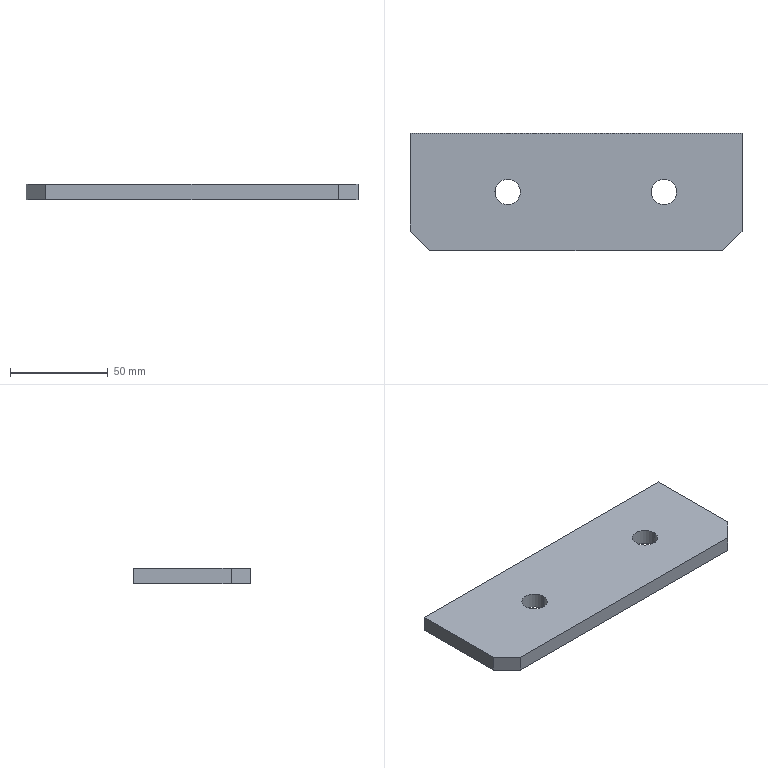Part | SolidWorks | features Extrusion 1, ICE 1 | 1 solid | 12 faces | box 170 x 60 x 8 mm | volume 78676 mm3 | plane 8 | cylinder 4 | commonest cylinder face diameters 13 x4
STEP:
#1=CARTESIAN_POINT('',(123.5,30.,0.));
#2=VERTEX_POINT('',#1);
#3=CARTESIAN_POINT('',(136.5,30.,0.));
#4=VERTEX_POINT('',#3);
#5=CARTESIAN_POINT('',(130.,30.,0.));
#6=DIRECTION('',(0.,0.,1.));
#7=DIRECTION('',(1.,0.,0.));
#8=AXIS2_PLACEMENT_3D('',#5,#6,#7);
#9=CIRCLE('',#8,6.5);
#10=EDGE_CURVE('',#2,#4,#9,.T.);
#11=ORIENTED_EDGE('',*,*,#10,.F.);
#12=CARTESIAN_POINT('',(123.5,30.,8.));
#13=VERTEX_POINT('',#12);
#14=CARTESIAN_POINT('',(123.5,30.,0.));
#15=DIRECTION('',(0.,0.,1.));
#16=VECTOR('',#15,1000.);
#17=LINE('',#14,#16);
#18=EDGE_CURVE('',#2,#13,#17,.T.);
#19=ORIENTED_EDGE('',*,*,#18,.T.);
#20=CARTESIAN_POINT('',(136.5,30.,8.));
#21=VERTEX_POINT('',#20);
#22=CARTESIAN_POINT('',(130.,30.,8.));
#23=DIRECTION('',(0.,0.,1.));
#24=DIRECTION('',(1.,0.,0.));
#25=AXIS2_PLACEMENT_3D('',#22,#23,#24);
#26=CIRCLE('',#25,6.5);
#27=EDGE_CURVE('',#13,#21,#26,.T.);
#28=ORIENTED_EDGE('',*,*,#27,.T.);
#29=CARTESIAN_POINT('',(136.5,30.,0.));
#30=DIRECTION('',(0.,0.,1.));
#31=VECTOR('',#30,1000.);
#32=LINE('',#29,#31);
#33=EDGE_CURVE('',#4,#21,#32,.T.);
#34=ORIENTED_EDGE('',*,*,#33,.F.);
#35=EDGE_LOOP('',(#11,#19,#28,#34));
#36=FACE_OUTER_BOUND('',#35,.T.);
#37=CARTESIAN_POINT('',(130.,30.,0.));
#38=DIRECTION('',(0.,0.,1.));
#39=DIRECTION('',(1.,0.,0.));
#40=AXIS2_PLACEMENT_3D('',#37,#38,#39);
#41=CYLINDRICAL_SURFACE('',#40,6.5);
#42=ADVANCED_FACE('',(#36),#41,.F.);
#43=CARTESIAN_POINT('',(43.5,30.,0.));
#44=VERTEX_POINT('',#43);
#45=CARTESIAN_POINT('',(56.5,30.,0.));
#46=VERTEX_POINT('',#45);
#47=CARTESIAN_POINT('',(50.,30.,0.));
#48=DIRECTION('',(0.,0.,1.));
#49=DIRECTION('',(1.,0.,0.));
#50=AXIS2_PLACEMENT_3D('',#47,#48,#49);
#51=CIRCLE('',#50,6.5);
#52=EDGE_CURVE('',#44,#46,#51,.T.);
#53=ORIENTED_EDGE('',*,*,#52,.F.);
#54=CARTESIAN_POINT('',(43.5,30.,8.));
#55=VERTEX_POINT('',#54);
#56=CARTESIAN_POINT('',(43.5,30.,0.));
#57=DIRECTION('',(0.,0.,1.));
#58=VECTOR('',#57,1000.);
#59=LINE('',#56,#58);
#60=EDGE_CURVE('',#44,#55,#59,.T.);
#61=ORIENTED_EDGE('',*,*,#60,.T.);
#62=CARTESIAN_POINT('',(56.5,30.,8.));
#63=VERTEX_POINT('',#62);
#64=CARTESIAN_POINT('',(50.,30.,8.));
#65=DIRECTION('',(0.,0.,1.));
#66=DIRECTION('',(1.,0.,0.));
#67=AXIS2_PLACEMENT_3D('',#64,#65,#66);
#68=CIRCLE('',#67,6.5);
#69=EDGE_CURVE('',#55,#63,#68,.T.);
#70=ORIENTED_EDGE('',*,*,#69,.T.);
#71=CARTESIAN_POINT('',(56.5,30.,0.));
#72=DIRECTION('',(0.,0.,1.));
#73=VECTOR('',#72,1000.);
#74=LINE('',#71,#73);
#75=EDGE_CURVE('',#46,#63,#74,.T.);
#76=ORIENTED_EDGE('',*,*,#75,.F.);
#77=EDGE_LOOP('',(#53,#61,#70,#76));
#78=FACE_OUTER_BOUND('',#77,.T.);
#79=CARTESIAN_POINT('',(50.,30.,0.));
#80=DIRECTION('',(0.,0.,1.));
#81=DIRECTION('',(1.,0.,0.));
#82=AXIS2_PLACEMENT_3D('',#79,#80,#81);
#83=CYLINDRICAL_SURFACE('',#82,6.5);
#84=ADVANCED_FACE('',(#78),#83,.F.);
#85=CARTESIAN_POINT('',(170.,60.,0.));
#86=VERTEX_POINT('',#85);
#87=CARTESIAN_POINT('',(0.,60.,0.));
#88=VERTEX_POINT('',#87);
#89=CARTESIAN_POINT('',(170.,60.,0.));
#90=DIRECTION('',(-1.,0.,0.));
#91=VECTOR('',#90,1000.);
#92=LINE('',#89,#91);
#93=EDGE_CURVE('',#86,#88,#92,.T.);
#94=ORIENTED_EDGE('',*,*,#93,.T.);
#95=CARTESIAN_POINT('',(0.,60.,8.));
#96=VERTEX_POINT('',#95);
#97=CARTESIAN_POINT('',(0.,60.,8.));
#98=DIRECTION('',(0.,0.,-1.));
#99=VECTOR('',#98,1000.);
#100=LINE('',#97,#99);
#101=EDGE_CURVE('',#96,#88,#100,.T.);
#102=ORIENTED_EDGE('',*,*,#101,.F.);
#103=CARTESIAN_POINT('',(170.,60.,8.));
#104=VERTEX_POINT('',#103);
#105=CARTESIAN_POINT('',(170.,60.,8.));
#106=DIRECTION('',(-1.,0.,0.));
#107=VECTOR('',#106,1000.);
#108=LINE('',#105,#107);
#109=EDGE_CURVE('',#104,#96,#108,.T.);
#110=ORIENTED_EDGE('',*,*,#109,.F.);
#111=CARTESIAN_POINT('',(170.,60.,8.));
#112=DIRECTION('',(0.,0.,-1.));
#113=VECTOR('',#112,1000.);
#114=LINE('',#111,#113);
#115=EDGE_CURVE('',#104,#86,#114,.T.);
#116=ORIENTED_EDGE('',*,*,#115,.T.);
#117=EDGE_LOOP('',(#94,#102,#110,#116));
#118=FACE_OUTER_BOUND('',#117,.T.);
#119=CARTESIAN_POINT('',(170.,60.,8.));
#120=DIRECTION('',(0.,-1.,0.));
#121=DIRECTION('',(0.,0.,-1.));
#122=AXIS2_PLACEMENT_3D('',#119,#120,#121);
#123=PLANE('',#122);
#124=ADVANCED_FACE('',(#118),#123,.F.);
#125=CARTESIAN_POINT('',(0.,10.,0.));
#126=VERTEX_POINT('',#125);
#127=CARTESIAN_POINT('',(0.,60.,0.));
#128=DIRECTION('',(0.,-1.,0.));
#129=VECTOR('',#128,1000.);
#130=LINE('',#127,#129);
#131=EDGE_CURVE('',#88,#126,#130,.T.);
#132=ORIENTED_EDGE('',*,*,#131,.T.);
#133=CARTESIAN_POINT('',(0.,10.,8.));
#134=VERTEX_POINT('',#133);
#135=CARTESIAN_POINT('',(0.,10.,8.));
#136=DIRECTION('',(0.,0.,-1.));
#137=VECTOR('',#136,1000.);
#138=LINE('',#135,#137);
#139=EDGE_CURVE('',#134,#126,#138,.T.);
#140=ORIENTED_EDGE('',*,*,#139,.F.);
#141=CARTESIAN_POINT('',(0.,60.,8.));
#142=DIRECTION('',(0.,-1.,0.));
#143=VECTOR('',#142,1000.);
#144=LINE('',#141,#143);
#145=EDGE_CURVE('',#96,#134,#144,.T.);
#146=ORIENTED_EDGE('',*,*,#145,.F.);
#147=ORIENTED_EDGE('',*,*,#101,.T.);
#148=EDGE_LOOP('',(#132,#140,#146,#147));
#149=FACE_OUTER_BOUND('',#148,.T.);
#150=CARTESIAN_POINT('',(0.,60.,8.));
#151=DIRECTION('',(1.,0.,0.));
#152=DIRECTION('',(0.,0.,-1.));
#153=AXIS2_PLACEMENT_3D('',#150,#151,#152);
#154=PLANE('',#153);
#155=ADVANCED_FACE('',(#149),#154,.F.);
#156=CARTESIAN_POINT('',(10.,0.,0.));
#157=VERTEX_POINT('',#156);
#158=CARTESIAN_POINT('',(0.,10.,0.));
#159=DIRECTION('',(0.7071,-0.7071,0.));
#160=VECTOR('',#159,1000.);
#161=LINE('',#158,#160);
#162=EDGE_CURVE('',#126,#157,#161,.T.);
#163=ORIENTED_EDGE('',*,*,#162,.T.);
#164=CARTESIAN_POINT('',(10.,0.,8.));
#165=VERTEX_POINT('',#164);
#166=CARTESIAN_POINT('',(10.,0.,8.));
#167=DIRECTION('',(0.,0.,-1.));
#168=VECTOR('',#167,1000.);
#169=LINE('',#166,#168);
#170=EDGE_CURVE('',#165,#157,#169,.T.);
#171=ORIENTED_EDGE('',*,*,#170,.F.);
#172=CARTESIAN_POINT('',(0.,10.,8.));
#173=DIRECTION('',(0.7071,-0.7071,0.));
#174=VECTOR('',#173,1000.);
#175=LINE('',#172,#174);
#176=EDGE_CURVE('',#134,#165,#175,.T.);
#177=ORIENTED_EDGE('',*,*,#176,.F.);
#178=ORIENTED_EDGE('',*,*,#139,.T.);
#179=EDGE_LOOP('',(#163,#171,#177,#178));
#180=FACE_OUTER_BOUND('',#179,.T.);
#181=CARTESIAN_POINT('',(0.,10.,8.));
#182=DIRECTION('',(0.7071,0.7071,0.));
#183=DIRECTION('',(-0.7071,0.7071,0.));
#184=AXIS2_PLACEMENT_3D('',#181,#182,#183);
#185=PLANE('',#184);
#186=ADVANCED_FACE('',(#180),#185,.F.);
#187=CARTESIAN_POINT('',(160.,0.,0.));
#188=VERTEX_POINT('',#187);
#189=CARTESIAN_POINT('',(10.,0.,0.));
#190=DIRECTION('',(1.,0.,0.));
#191=VECTOR('',#190,1000.);
#192=LINE('',#189,#191);
#193=EDGE_CURVE('',#157,#188,#192,.T.);
#194=ORIENTED_EDGE('',*,*,#193,.T.);
#195=CARTESIAN_POINT('',(160.,0.,8.));
#196=VERTEX_POINT('',#195);
#197=CARTESIAN_POINT('',(160.,0.,8.));
#198=DIRECTION('',(0.,0.,-1.));
#199=VECTOR('',#198,1000.);
#200=LINE('',#197,#199);
#201=EDGE_CURVE('',#196,#188,#200,.T.);
#202=ORIENTED_EDGE('',*,*,#201,.F.);
#203=CARTESIAN_POINT('',(10.,0.,8.));
#204=DIRECTION('',(1.,0.,0.));
#205=VECTOR('',#204,1000.);
#206=LINE('',#203,#205);
#207=EDGE_CURVE('',#165,#196,#206,.T.);
#208=ORIENTED_EDGE('',*,*,#207,.F.);
#209=ORIENTED_EDGE('',*,*,#170,.T.);
#210=EDGE_LOOP('',(#194,#202,#208,#209));
#211=FACE_OUTER_BOUND('',#210,.T.);
#212=CARTESIAN_POINT('',(10.,0.,8.));
#213=DIRECTION('',(0.,1.,0.));
#214=DIRECTION('',(0.,0.,1.));
#215=AXIS2_PLACEMENT_3D('',#212,#213,#214);
#216=PLANE('',#215);
#217=ADVANCED_FACE('',(#211),#216,.F.);
#218=CARTESIAN_POINT('',(170.,10.,0.));
#219=VERTEX_POINT('',#218);
#220=CARTESIAN_POINT('',(160.,0.,0.));
#221=DIRECTION('',(0.7071,0.7071,0.));
#222=VECTOR('',#221,1000.);
#223=LINE('',#220,#222);
#224=EDGE_CURVE('',#188,#219,#223,.T.);
#225=ORIENTED_EDGE('',*,*,#224,.T.);
#226=CARTESIAN_POINT('',(170.,10.,8.));
#227=VERTEX_POINT('',#226);
#228=CARTESIAN_POINT('',(170.,10.,8.));
#229=DIRECTION('',(0.,0.,-1.));
#230=VECTOR('',#229,1000.);
#231=LINE('',#228,#230);
#232=EDGE_CURVE('',#227,#219,#231,.T.);
#233=ORIENTED_EDGE('',*,*,#232,.F.);
#234=CARTESIAN_POINT('',(160.,0.,8.));
#235=DIRECTION('',(0.7071,0.7071,0.));
#236=VECTOR('',#235,1000.);
#237=LINE('',#234,#236);
#238=EDGE_CURVE('',#196,#227,#237,.T.);
#239=ORIENTED_EDGE('',*,*,#238,.F.);
#240=ORIENTED_EDGE('',*,*,#201,.T.);
#241=EDGE_LOOP('',(#225,#233,#239,#240));
#242=FACE_OUTER_BOUND('',#241,.T.);
#243=CARTESIAN_POINT('',(160.,0.,8.));
#244=DIRECTION('',(-0.7071,0.7071,0.));
#245=DIRECTION('',(-0.7071,-0.7071,0.));
#246=AXIS2_PLACEMENT_3D('',#243,#244,#245);
#247=PLANE('',#246);
#248=ADVANCED_FACE('',(#242),#247,.F.);
#249=CARTESIAN_POINT('',(170.,10.,0.));
#250=DIRECTION('',(0.,1.,0.));
#251=VECTOR('',#250,1000.);
#252=LINE('',#249,#251);
#253=EDGE_CURVE('',#219,#86,#252,.T.);
#254=ORIENTED_EDGE('',*,*,#253,.T.);
#255=ORIENTED_EDGE('',*,*,#115,.F.);
#256=CARTESIAN_POINT('',(170.,10.,8.));
#257=DIRECTION('',(0.,1.,0.));
#258=VECTOR('',#257,1000.);
#259=LINE('',#256,#258);
#260=EDGE_CURVE('',#227,#104,#259,.T.);
#261=ORIENTED_EDGE('',*,*,#260,.F.);
#262=ORIENTED_EDGE('',*,*,#232,.T.);
#263=EDGE_LOOP('',(#254,#255,#261,#262));
#264=FACE_OUTER_BOUND('',#263,.T.);
#265=CARTESIAN_POINT('',(170.,10.,8.));
#266=DIRECTION('',(-1.,0.,0.));
#267=DIRECTION('',(0.,0.,1.));
#268=AXIS2_PLACEMENT_3D('',#265,#266,#267);
#269=PLANE('',#268);
#270=ADVANCED_FACE('',(#264),#269,.F.);
#271=CARTESIAN_POINT('',(130.,30.,8.));
#272=DIRECTION('',(0.,0.,1.));
#273=DIRECTION('',(1.,0.,0.));
#274=AXIS2_PLACEMENT_3D('',#271,#272,#273);
#275=CIRCLE('',#274,6.5);
#276=EDGE_CURVE('',#21,#13,#275,.T.);
#277=ORIENTED_EDGE('',*,*,#276,.F.);
#278=ORIENTED_EDGE('',*,*,#27,.F.);
#279=EDGE_LOOP('',(#277,#278));
#280=FACE_BOUND('',#279,.T.);
#281=CARTESIAN_POINT('',(50.,30.,8.));
#282=DIRECTION('',(0.,0.,1.));
#283=DIRECTION('',(1.,0.,0.));
#284=AXIS2_PLACEMENT_3D('',#281,#282,#283);
#285=CIRCLE('',#284,6.5);
#286=EDGE_CURVE('',#63,#55,#285,.T.);
#287=ORIENTED_EDGE('',*,*,#286,.F.);
#288=ORIENTED_EDGE('',*,*,#69,.F.);
#289=EDGE_LOOP('',(#287,#288));
#290=FACE_BOUND('',#289,.T.);
#291=ORIENTED_EDGE('',*,*,#109,.T.);
#292=ORIENTED_EDGE('',*,*,#145,.T.);
#293=ORIENTED_EDGE('',*,*,#176,.T.);
#294=ORIENTED_EDGE('',*,*,#207,.T.);
#295=ORIENTED_EDGE('',*,*,#238,.T.);
#296=ORIENTED_EDGE('',*,*,#260,.T.);
#297=EDGE_LOOP('',(#291,#292,#293,#294,#295,#296));
#298=FACE_OUTER_BOUND('',#297,.T.);
#299=CARTESIAN_POINT('',(0.,0.,8.));
#300=DIRECTION('',(0.,0.,1.));
#301=DIRECTION('',(1.,0.,0.));
#302=AXIS2_PLACEMENT_3D('',#299,#300,#301);
#303=PLANE('',#302);
#304=ADVANCED_FACE('',(#280,#290,#298),#303,.T.);
#305=CARTESIAN_POINT('',(130.,30.,0.));
#306=DIRECTION('',(0.,0.,1.));
#307=DIRECTION('',(1.,0.,0.));
#308=AXIS2_PLACEMENT_3D('',#305,#306,#307);
#309=CIRCLE('',#308,6.5);
#310=EDGE_CURVE('',#4,#2,#309,.T.);
#311=ORIENTED_EDGE('',*,*,#310,.T.);
#312=ORIENTED_EDGE('',*,*,#10,.T.);
#313=EDGE_LOOP('',(#311,#312));
#314=FACE_BOUND('',#313,.T.);
#315=CARTESIAN_POINT('',(50.,30.,0.));
#316=DIRECTION('',(0.,0.,1.));
#317=DIRECTION('',(1.,0.,0.));
#318=AXIS2_PLACEMENT_3D('',#315,#316,#317);
#319=CIRCLE('',#318,6.5);
#320=EDGE_CURVE('',#46,#44,#319,.T.);
#321=ORIENTED_EDGE('',*,*,#320,.T.);
#322=ORIENTED_EDGE('',*,*,#52,.T.);
#323=EDGE_LOOP('',(#321,#322));
#324=FACE_BOUND('',#323,.T.);
#325=ORIENTED_EDGE('',*,*,#93,.F.);
#326=ORIENTED_EDGE('',*,*,#253,.F.);
#327=ORIENTED_EDGE('',*,*,#224,.F.);
#328=ORIENTED_EDGE('',*,*,#193,.F.);
#329=ORIENTED_EDGE('',*,*,#162,.F.);
#330=ORIENTED_EDGE('',*,*,#131,.F.);
#331=EDGE_LOOP('',(#325,#326,#327,#328,#329,#330));
#332=FACE_OUTER_BOUND('',#331,.T.);
#333=CARTESIAN_POINT('',(0.,0.,0.));
#334=DIRECTION('',(0.,0.,1.));
#335=DIRECTION('',(1.,0.,0.));
#336=AXIS2_PLACEMENT_3D('',#333,#334,#335);
#337=PLANE('',#336);
#338=ADVANCED_FACE('',(#314,#324,#332),#337,.F.);
#339=ORIENTED_EDGE('',*,*,#60,.F.);
#340=ORIENTED_EDGE('',*,*,#320,.F.);
#341=ORIENTED_EDGE('',*,*,#75,.T.);
#342=ORIENTED_EDGE('',*,*,#286,.T.);
#343=EDGE_LOOP('',(#339,#340,#341,#342));
#344=FACE_OUTER_BOUND('',#343,.T.);
#345=CARTESIAN_POINT('',(50.,30.,0.));
#346=DIRECTION('',(0.,0.,1.));
#347=DIRECTION('',(1.,0.,0.));
#348=AXIS2_PLACEMENT_3D('',#345,#346,#347);
#349=CYLINDRICAL_SURFACE('',#348,6.5);
#350=ADVANCED_FACE('',(#344),#349,.F.);
#351=ORIENTED_EDGE('',*,*,#18,.F.);
#352=ORIENTED_EDGE('',*,*,#310,.F.);
#353=ORIENTED_EDGE('',*,*,#33,.T.);
#354=ORIENTED_EDGE('',*,*,#276,.T.);
#355=EDGE_LOOP('',(#351,#352,#353,#354));
#356=FACE_OUTER_BOUND('',#355,.T.);
#357=CARTESIAN_POINT('',(130.,30.,0.));
#358=DIRECTION('',(0.,0.,1.));
#359=DIRECTION('',(1.,0.,0.));
#360=AXIS2_PLACEMENT_3D('',#357,#358,#359);
#361=CYLINDRICAL_SURFACE('',#360,6.5);
#362=ADVANCED_FACE('',(#356),#361,.F.);
#363=CLOSED_SHELL('',(#42,#84,#124,#155,#186,#217,#248,#270,#304,#338,#350,#362));
#364=MANIFOLD_SOLID_BREP('',#363);
#365=CARTESIAN_POINT('',(0.,0.,0.));
#366=DIRECTION('',(0.,0.,1.));
#367=DIRECTION('',(1.,0.,0.));
#368=AXIS2_PLACEMENT_3D('',#365,#366,#367);
#369=(LENGTH_UNIT()NAMED_UNIT(*)SI_UNIT(.MILLI.,.METRE.));
#370=UNCERTAINTY_MEASURE_WITH_UNIT(LENGTH_MEASURE(0.00001),#369,'','');
#371=(NAMED_UNIT(*)PLANE_ANGLE_UNIT()SI_UNIT($,.RADIAN.));
#372=(NAMED_UNIT(*)SI_UNIT($,.STERADIAN.)SOLID_ANGLE_UNIT());
#373=(GEOMETRIC_REPRESENTATION_CONTEXT(3)GLOBAL_UNCERTAINTY_ASSIGNED_CONTEXT((#370))GLOBAL_UNIT_ASSIGNED_CONTEXT((#369,#371,#372))REPRESENTATION_CONTEXT('',''));
#374=ADVANCED_BREP_SHAPE_REPRESENTATION('',(#364,#368),#373);